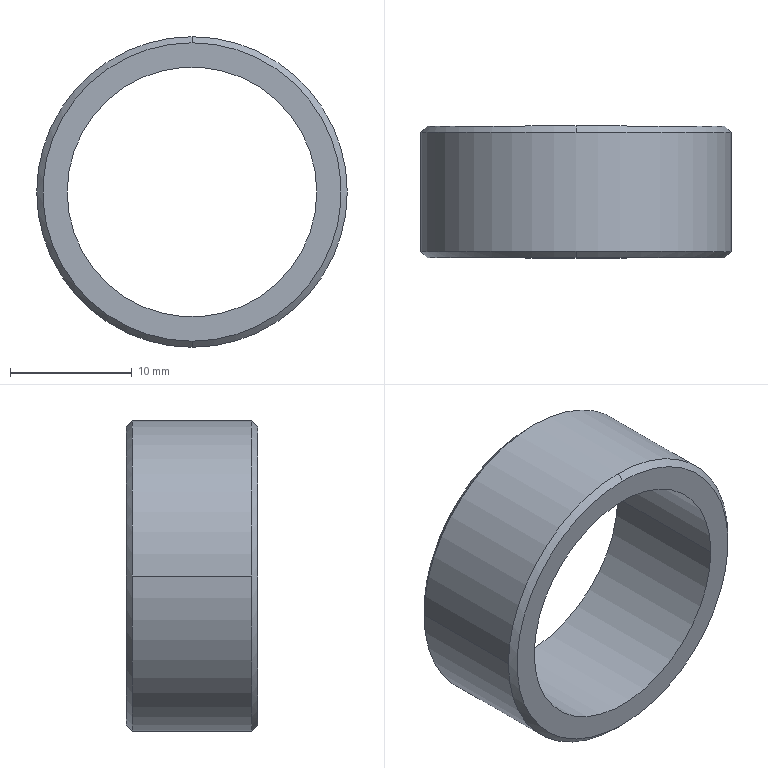Part | SolidWorks | features BaseBody 1 | 1 solid | 10 faces | box 25.5 x 10.8 x 25.5 mm | volume 1931 mm3 | cone 4 | cylinder 4 | plane 2 | commonest cylinder face diameters 20.5 x2 25.5 x2
STEP:
#1=CARTESIAN_POINT('',(624.451,57.35,30.033));
#2=VERTEX_POINT('',#1);
#3=CARTESIAN_POINT('',(624.451,57.35,5.533));
#4=VERTEX_POINT('',#3);
#5=CARTESIAN_POINT('',(624.451,57.35,17.783));
#6=DIRECTION('',(0.,-1.,0.));
#7=DIRECTION('',(0.,0.,-1.));
#8=AXIS2_PLACEMENT_3D('',#5,#6,#7);
#9=CIRCLE('',#8,12.25);
#10=EDGE_CURVE('',#2,#4,#9,.T.);
#11=ORIENTED_EDGE('',*,*,#10,.F.);
#12=CARTESIAN_POINT('',(624.451,57.85,30.533));
#13=VERTEX_POINT('',#12);
#14=CARTESIAN_POINT('',(624.451,57.35,30.033));
#15=DIRECTION('',(0.,0.7071,0.7071));
#16=VECTOR('',#15,1000.);
#17=LINE('',#14,#16);
#18=EDGE_CURVE('',#2,#13,#17,.T.);
#19=ORIENTED_EDGE('',*,*,#18,.T.);
#20=CARTESIAN_POINT('',(611.701,57.85,17.783));
#21=VERTEX_POINT('',#20);
#22=CARTESIAN_POINT('',(624.451,57.85,17.783));
#23=DIRECTION('',(0.,1.,0.));
#24=DIRECTION('',(0.,0.,1.));
#25=AXIS2_PLACEMENT_3D('',#22,#23,#24);
#26=CIRCLE('',#25,12.75);
#27=EDGE_CURVE('',#21,#13,#26,.T.);
#28=ORIENTED_EDGE('',*,*,#27,.F.);
#29=CARTESIAN_POINT('',(624.451,57.85,5.033));
#30=VERTEX_POINT('',#29);
#31=CARTESIAN_POINT('',(624.451,57.85,17.783));
#32=DIRECTION('',(0.,1.,0.));
#33=DIRECTION('',(0.,0.,1.));
#34=AXIS2_PLACEMENT_3D('',#31,#32,#33);
#35=CIRCLE('',#34,12.75);
#36=EDGE_CURVE('',#30,#21,#35,.T.);
#37=ORIENTED_EDGE('',*,*,#36,.F.);
#38=CARTESIAN_POINT('',(624.451,57.35,5.533));
#39=DIRECTION('',(0.,0.7071,-0.7071));
#40=VECTOR('',#39,1000.);
#41=LINE('',#38,#40);
#42=EDGE_CURVE('',#4,#30,#41,.T.);
#43=ORIENTED_EDGE('',*,*,#42,.F.);
#44=EDGE_LOOP('',(#11,#19,#28,#37,#43));
#45=FACE_OUTER_BOUND('',#44,.T.);
#46=CARTESIAN_POINT('',(624.451,57.35,17.783));
#47=DIRECTION('',(0.,1.,0.));
#48=DIRECTION('',(0.,0.,-1.));
#49=AXIS2_PLACEMENT_3D('',#46,#47,#48);
#50=CONICAL_SURFACE('',#49,12.25,0.7854);
#51=ADVANCED_FACE('',(#45),#50,.T.);
#52=CARTESIAN_POINT('',(624.451,68.15,5.533));
#53=VERTEX_POINT('',#52);
#54=CARTESIAN_POINT('',(624.451,68.15,30.033));
#55=VERTEX_POINT('',#54);
#56=CARTESIAN_POINT('',(624.451,68.15,17.783));
#57=DIRECTION('',(0.,1.,0.));
#58=DIRECTION('',(0.,0.,1.));
#59=AXIS2_PLACEMENT_3D('',#56,#57,#58);
#60=CIRCLE('',#59,12.25);
#61=EDGE_CURVE('',#53,#55,#60,.T.);
#62=ORIENTED_EDGE('',*,*,#61,.F.);
#63=CARTESIAN_POINT('',(624.451,67.65,5.033));
#64=VERTEX_POINT('',#63);
#65=CARTESIAN_POINT('',(624.451,67.65,5.033));
#66=DIRECTION('',(0.,-0.7071,-0.7071));
#67=VECTOR('',#66,1000.);
#68=LINE('',#65,#67);
#69=EDGE_CURVE('',#53,#64,#68,.T.);
#70=ORIENTED_EDGE('',*,*,#69,.T.);
#71=CARTESIAN_POINT('',(611.701,67.65,17.783));
#72=VERTEX_POINT('',#71);
#73=CARTESIAN_POINT('',(624.451,67.65,17.783));
#74=DIRECTION('',(0.,-1.,0.));
#75=DIRECTION('',(0.,0.,-1.));
#76=AXIS2_PLACEMENT_3D('',#73,#74,#75);
#77=CIRCLE('',#76,12.75);
#78=EDGE_CURVE('',#72,#64,#77,.T.);
#79=ORIENTED_EDGE('',*,*,#78,.F.);
#80=CARTESIAN_POINT('',(624.451,67.65,30.533));
#81=VERTEX_POINT('',#80);
#82=CARTESIAN_POINT('',(624.451,67.65,17.783));
#83=DIRECTION('',(0.,-1.,0.));
#84=DIRECTION('',(0.,0.,-1.));
#85=AXIS2_PLACEMENT_3D('',#82,#83,#84);
#86=CIRCLE('',#85,12.75);
#87=EDGE_CURVE('',#81,#72,#86,.T.);
#88=ORIENTED_EDGE('',*,*,#87,.F.);
#89=CARTESIAN_POINT('',(624.451,67.65,30.533));
#90=DIRECTION('',(0.,-0.7071,0.7071));
#91=VECTOR('',#90,1000.);
#92=LINE('',#89,#91);
#93=EDGE_CURVE('',#55,#81,#92,.T.);
#94=ORIENTED_EDGE('',*,*,#93,.F.);
#95=EDGE_LOOP('',(#62,#70,#79,#88,#94));
#96=FACE_OUTER_BOUND('',#95,.T.);
#97=CARTESIAN_POINT('',(624.451,67.65,17.783));
#98=DIRECTION('',(0.,-1.,0.));
#99=DIRECTION('',(0.,0.,1.));
#100=AXIS2_PLACEMENT_3D('',#97,#98,#99);
#101=CONICAL_SURFACE('',#100,12.75,0.7854);
#102=ADVANCED_FACE('',(#96),#101,.T.);
#103=CARTESIAN_POINT('',(634.701,68.15,17.783));
#104=VERTEX_POINT('',#103);
#105=CARTESIAN_POINT('',(614.201,68.15,17.783));
#106=VERTEX_POINT('',#105);
#107=CARTESIAN_POINT('',(624.451,68.15,17.783));
#108=DIRECTION('',(0.,-1.,0.));
#109=DIRECTION('',(0.,0.,1.));
#110=AXIS2_PLACEMENT_3D('',#107,#108,#109);
#111=CIRCLE('',#110,10.25);
#112=EDGE_CURVE('',#104,#106,#111,.T.);
#113=ORIENTED_EDGE('',*,*,#112,.F.);
#114=CARTESIAN_POINT('',(634.701,57.35,17.783));
#115=VERTEX_POINT('',#114);
#116=CARTESIAN_POINT('',(634.701,72.25,17.783));
#117=DIRECTION('',(0.,-1.,0.));
#118=VECTOR('',#117,1000.);
#119=LINE('',#116,#118);
#120=EDGE_CURVE('',#104,#115,#119,.T.);
#121=ORIENTED_EDGE('',*,*,#120,.T.);
#122=CARTESIAN_POINT('',(614.201,57.35,17.783));
#123=VERTEX_POINT('',#122);
#124=CARTESIAN_POINT('',(624.451,57.35,17.783));
#125=DIRECTION('',(0.,-1.,0.));
#126=DIRECTION('',(0.,0.,-1.));
#127=AXIS2_PLACEMENT_3D('',#124,#125,#126);
#128=CIRCLE('',#127,10.25);
#129=EDGE_CURVE('',#115,#123,#128,.T.);
#130=ORIENTED_EDGE('',*,*,#129,.T.);
#131=CARTESIAN_POINT('',(614.201,72.25,17.783));
#132=DIRECTION('',(0.,-1.,0.));
#133=VECTOR('',#132,1000.);
#134=LINE('',#131,#133);
#135=EDGE_CURVE('',#106,#123,#134,.T.);
#136=ORIENTED_EDGE('',*,*,#135,.F.);
#137=EDGE_LOOP('',(#113,#121,#130,#136));
#138=FACE_OUTER_BOUND('',#137,.T.);
#139=CARTESIAN_POINT('',(624.451,72.25,17.783));
#140=DIRECTION('',(0.,-1.,0.));
#141=DIRECTION('',(-1.,0.,0.));
#142=AXIS2_PLACEMENT_3D('',#139,#140,#141);
#143=CYLINDRICAL_SURFACE('',#142,10.25);
#144=ADVANCED_FACE('',(#138),#143,.F.);
#145=ORIENTED_EDGE('',*,*,#78,.T.);
#146=CARTESIAN_POINT('',(637.201,67.65,17.783));
#147=VERTEX_POINT('',#146);
#148=CARTESIAN_POINT('',(624.451,67.65,17.783));
#149=DIRECTION('',(0.,-1.,0.));
#150=DIRECTION('',(0.,0.,-1.));
#151=AXIS2_PLACEMENT_3D('',#148,#149,#150);
#152=CIRCLE('',#151,12.75);
#153=EDGE_CURVE('',#64,#147,#152,.T.);
#154=ORIENTED_EDGE('',*,*,#153,.T.);
#155=CARTESIAN_POINT('',(637.201,57.85,17.783));
#156=VERTEX_POINT('',#155);
#157=CARTESIAN_POINT('',(637.201,72.25,17.783));
#158=DIRECTION('',(0.,-1.,0.));
#159=VECTOR('',#158,1000.);
#160=LINE('',#157,#159);
#161=EDGE_CURVE('',#147,#156,#160,.T.);
#162=ORIENTED_EDGE('',*,*,#161,.T.);
#163=CARTESIAN_POINT('',(624.451,57.85,17.783));
#164=DIRECTION('',(0.,1.,0.));
#165=DIRECTION('',(0.,0.,1.));
#166=AXIS2_PLACEMENT_3D('',#163,#164,#165);
#167=CIRCLE('',#166,12.75);
#168=EDGE_CURVE('',#156,#30,#167,.T.);
#169=ORIENTED_EDGE('',*,*,#168,.T.);
#170=ORIENTED_EDGE('',*,*,#36,.T.);
#171=CARTESIAN_POINT('',(611.701,72.25,17.783));
#172=DIRECTION('',(0.,-1.,0.));
#173=VECTOR('',#172,1000.);
#174=LINE('',#171,#173);
#175=EDGE_CURVE('',#72,#21,#174,.T.);
#176=ORIENTED_EDGE('',*,*,#175,.F.);
#177=EDGE_LOOP('',(#145,#154,#162,#169,#170,#176));
#178=FACE_OUTER_BOUND('',#177,.T.);
#179=CARTESIAN_POINT('',(624.451,72.25,17.783));
#180=DIRECTION('',(0.,-1.,0.));
#181=DIRECTION('',(-1.,0.,0.));
#182=AXIS2_PLACEMENT_3D('',#179,#180,#181);
#183=CYLINDRICAL_SURFACE('',#182,12.75);
#184=ADVANCED_FACE('',(#178),#183,.T.);
#185=ORIENTED_EDGE('',*,*,#161,.F.);
#186=CARTESIAN_POINT('',(624.451,67.65,17.783));
#187=DIRECTION('',(0.,-1.,0.));
#188=DIRECTION('',(0.,0.,-1.));
#189=AXIS2_PLACEMENT_3D('',#186,#187,#188);
#190=CIRCLE('',#189,12.75);
#191=EDGE_CURVE('',#147,#81,#190,.T.);
#192=ORIENTED_EDGE('',*,*,#191,.T.);
#193=ORIENTED_EDGE('',*,*,#87,.T.);
#194=ORIENTED_EDGE('',*,*,#175,.T.);
#195=ORIENTED_EDGE('',*,*,#27,.T.);
#196=CARTESIAN_POINT('',(624.451,57.85,17.783));
#197=DIRECTION('',(0.,1.,0.));
#198=DIRECTION('',(0.,0.,1.));
#199=AXIS2_PLACEMENT_3D('',#196,#197,#198);
#200=CIRCLE('',#199,12.75);
#201=EDGE_CURVE('',#13,#156,#200,.T.);
#202=ORIENTED_EDGE('',*,*,#201,.T.);
#203=EDGE_LOOP('',(#185,#192,#193,#194,#195,#202));
#204=FACE_OUTER_BOUND('',#203,.T.);
#205=CARTESIAN_POINT('',(624.451,72.25,17.783));
#206=DIRECTION('',(0.,-1.,0.));
#207=DIRECTION('',(-1.,0.,0.));
#208=AXIS2_PLACEMENT_3D('',#205,#206,#207);
#209=CYLINDRICAL_SURFACE('',#208,12.75);
#210=ADVANCED_FACE('',(#204),#209,.T.);
#211=CARTESIAN_POINT('',(624.451,57.35,17.783));
#212=DIRECTION('',(0.,-1.,0.));
#213=DIRECTION('',(0.,0.,-1.));
#214=AXIS2_PLACEMENT_3D('',#211,#212,#213);
#215=CIRCLE('',#214,10.25);
#216=EDGE_CURVE('',#123,#115,#215,.T.);
#217=ORIENTED_EDGE('',*,*,#216,.F.);
#218=ORIENTED_EDGE('',*,*,#129,.F.);
#219=EDGE_LOOP('',(#217,#218));
#220=FACE_BOUND('',#219,.T.);
#221=CARTESIAN_POINT('',(624.451,57.35,17.783));
#222=DIRECTION('',(0.,-1.,0.));
#223=DIRECTION('',(0.,0.,-1.));
#224=AXIS2_PLACEMENT_3D('',#221,#222,#223);
#225=CIRCLE('',#224,12.25);
#226=EDGE_CURVE('',#4,#2,#225,.T.);
#227=ORIENTED_EDGE('',*,*,#226,.T.);
#228=ORIENTED_EDGE('',*,*,#10,.T.);
#229=EDGE_LOOP('',(#227,#228));
#230=FACE_OUTER_BOUND('',#229,.T.);
#231=CARTESIAN_POINT('',(589.812,57.35,21.053));
#232=DIRECTION('',(0.,-1.,0.));
#233=DIRECTION('',(0.,0.,-1.));
#234=AXIS2_PLACEMENT_3D('',#231,#232,#233);
#235=PLANE('',#234);
#236=ADVANCED_FACE('',(#220,#230),#235,.T.);
#237=CARTESIAN_POINT('',(624.451,68.15,17.783));
#238=DIRECTION('',(0.,-1.,0.));
#239=DIRECTION('',(0.,0.,1.));
#240=AXIS2_PLACEMENT_3D('',#237,#238,#239);
#241=CIRCLE('',#240,10.25);
#242=EDGE_CURVE('',#106,#104,#241,.T.);
#243=ORIENTED_EDGE('',*,*,#242,.T.);
#244=ORIENTED_EDGE('',*,*,#112,.T.);
#245=EDGE_LOOP('',(#243,#244));
#246=FACE_BOUND('',#245,.T.);
#247=CARTESIAN_POINT('',(624.451,68.15,17.783));
#248=DIRECTION('',(0.,1.,0.));
#249=DIRECTION('',(0.,0.,1.));
#250=AXIS2_PLACEMENT_3D('',#247,#248,#249);
#251=CIRCLE('',#250,12.25);
#252=EDGE_CURVE('',#55,#53,#251,.T.);
#253=ORIENTED_EDGE('',*,*,#252,.T.);
#254=ORIENTED_EDGE('',*,*,#61,.T.);
#255=EDGE_LOOP('',(#253,#254));
#256=FACE_OUTER_BOUND('',#255,.T.);
#257=CARTESIAN_POINT('',(589.812,68.15,21.053));
#258=DIRECTION('',(0.,1.,0.));
#259=DIRECTION('',(1.,0.,0.));
#260=AXIS2_PLACEMENT_3D('',#257,#258,#259);
#261=PLANE('',#260);
#262=ADVANCED_FACE('',(#246,#256),#261,.T.);
#263=ORIENTED_EDGE('',*,*,#120,.F.);
#264=ORIENTED_EDGE('',*,*,#242,.F.);
#265=ORIENTED_EDGE('',*,*,#135,.T.);
#266=ORIENTED_EDGE('',*,*,#216,.T.);
#267=EDGE_LOOP('',(#263,#264,#265,#266));
#268=FACE_OUTER_BOUND('',#267,.T.);
#269=CARTESIAN_POINT('',(624.451,72.25,17.783));
#270=DIRECTION('',(0.,-1.,0.));
#271=DIRECTION('',(-1.,0.,0.));
#272=AXIS2_PLACEMENT_3D('',#269,#270,#271);
#273=CYLINDRICAL_SURFACE('',#272,10.25);
#274=ADVANCED_FACE('',(#268),#273,.F.);
#275=ORIENTED_EDGE('',*,*,#69,.F.);
#276=ORIENTED_EDGE('',*,*,#252,.F.);
#277=ORIENTED_EDGE('',*,*,#93,.T.);
#278=ORIENTED_EDGE('',*,*,#191,.F.);
#279=ORIENTED_EDGE('',*,*,#153,.F.);
#280=EDGE_LOOP('',(#275,#276,#277,#278,#279));
#281=FACE_OUTER_BOUND('',#280,.T.);
#282=CARTESIAN_POINT('',(624.451,67.65,17.783));
#283=DIRECTION('',(0.,-1.,0.));
#284=DIRECTION('',(0.,0.,1.));
#285=AXIS2_PLACEMENT_3D('',#282,#283,#284);
#286=CONICAL_SURFACE('',#285,12.75,0.7854);
#287=ADVANCED_FACE('',(#281),#286,.T.);
#288=ORIENTED_EDGE('',*,*,#18,.F.);
#289=ORIENTED_EDGE('',*,*,#226,.F.);
#290=ORIENTED_EDGE('',*,*,#42,.T.);
#291=ORIENTED_EDGE('',*,*,#168,.F.);
#292=ORIENTED_EDGE('',*,*,#201,.F.);
#293=EDGE_LOOP('',(#288,#289,#290,#291,#292));
#294=FACE_OUTER_BOUND('',#293,.T.);
#295=CARTESIAN_POINT('',(624.451,57.35,17.783));
#296=DIRECTION('',(0.,1.,0.));
#297=DIRECTION('',(0.,0.,-1.));
#298=AXIS2_PLACEMENT_3D('',#295,#296,#297);
#299=CONICAL_SURFACE('',#298,12.25,0.7854);
#300=ADVANCED_FACE('',(#294),#299,.T.);
#301=CLOSED_SHELL('',(#51,#102,#144,#184,#210,#236,#262,#274,#287,#300));
#302=MANIFOLD_SOLID_BREP('',#301);
#303=CARTESIAN_POINT('',(0.,0.,0.));
#304=DIRECTION('',(0.,0.,1.));
#305=DIRECTION('',(1.,0.,0.));
#306=AXIS2_PLACEMENT_3D('',#303,#304,#305);
#307=(LENGTH_UNIT()NAMED_UNIT(*)SI_UNIT(.MILLI.,.METRE.));
#308=UNCERTAINTY_MEASURE_WITH_UNIT(LENGTH_MEASURE(0.00001),#307,'','');
#309=(NAMED_UNIT(*)PLANE_ANGLE_UNIT()SI_UNIT($,.RADIAN.));
#310=(NAMED_UNIT(*)SI_UNIT($,.STERADIAN.)SOLID_ANGLE_UNIT());
#311=(GEOMETRIC_REPRESENTATION_CONTEXT(3)GLOBAL_UNCERTAINTY_ASSIGNED_CONTEXT((#308))GLOBAL_UNIT_ASSIGNED_CONTEXT((#307,#309,#310))REPRESENTATION_CONTEXT('',''));
#312=ADVANCED_BREP_SHAPE_REPRESENTATION('',(#302,#306),#311);